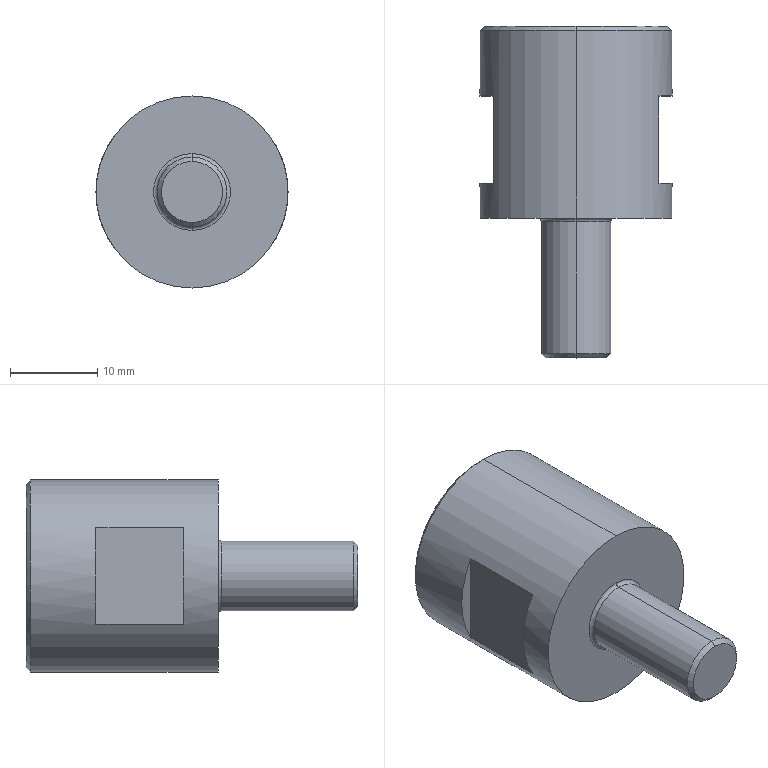Part | STEP file | OP10-142_seal rod plug | 1 solid | 34 faces | box 22 x 38 x 22 mm | volume 7650 mm3 | cylinder 13 | plane 11 | cone 8 | torus 2 | commonest cylinder face diameters 4 x5 8 x2 15.345 x2 16.5 x2 22 x2